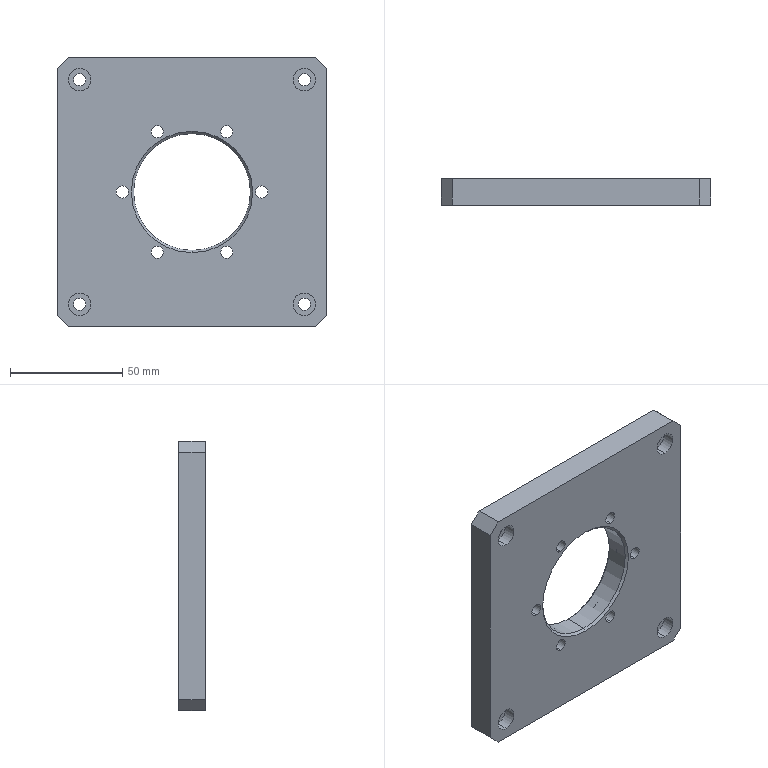Part | STEP file | ND25021-01-JDKM-67-TL | 1 solid | 66 faces | box 120 x 12 x 120 mm | volume 140750 mm3 | cylinder 42 | plane 20 | cone 4 | commonest cylinder face diameters 5.5 x20 9.999 x12 10 x8 52 x2